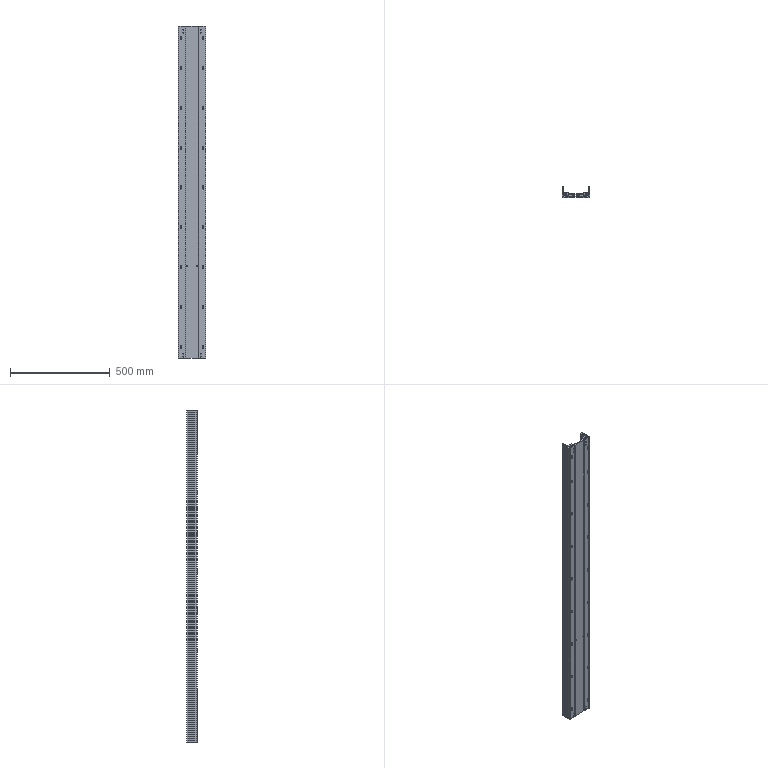Part | SolidWorks | features BaseBody 1 | 1 solid | 359 faces | box 140 x 53 x 1667 mm | volume 3998798 mm3 | cylinder 234 | plane 125 | commonest cylinder face diameters 5 x104 6.6 x36 11 x36 4 x16 3.3 x12 0.6 x8